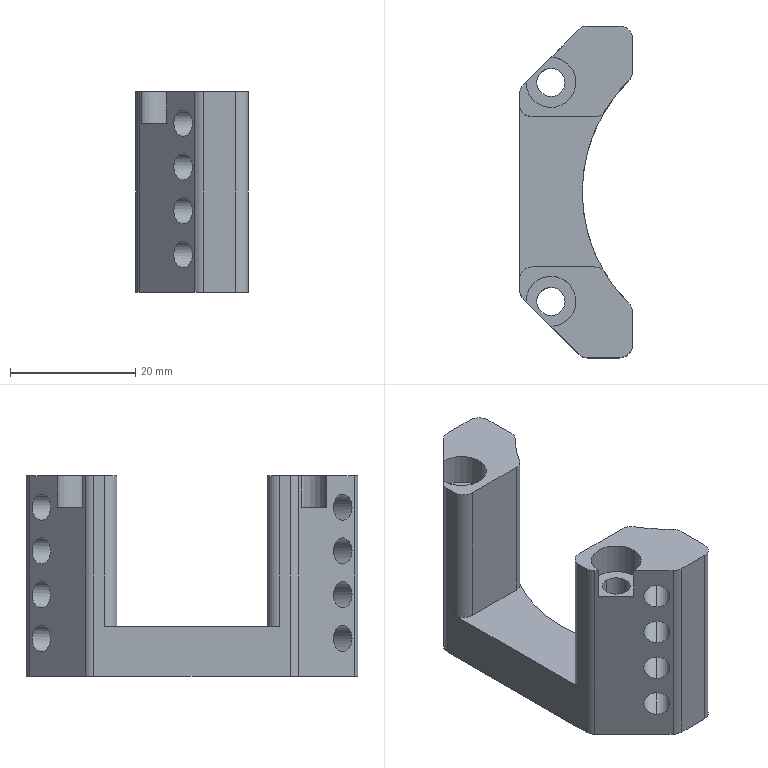NC program | Mastercam | posted with a generic post
Lines 42 to 1196 of 15624:
N430 T11 M6
N440 G0 G90 G17 G54 X-30.233 Y-26.319 A0. S7000 M3
N450 G43 H11 Z50. M8
N460 Z-22.696
N470 G1 Z-23.196 F600.
N480 X-30.432 Y-26.384 Z-23.233 F3000.
N490 X-30.636 Y-26.427 Z-23.27
N500 X-30.845 Y-26.449 Z-23.307
N510 X-31.054 Y-26.45 Z-23.344
N520 X-31.262 Y-26.428 Z-23.381
N530 X-31.467 Y-26.385 Z-23.418
N540 X-31.666 Y-26.32 Z-23.455
N550 X-31.857 Y-26.235 Z-23.491
N560 X-32.039 Y-26.131 Z-23.528
N570 X-32.208 Y-26.008 Z-23.565
N580 X-32.364 Y-25.868 Z-23.602
N590 X-32.504 Y-25.713 Z-23.639
N600 X-32.628 Y-25.543 Z-23.676
N610 X-32.732 Y-25.362 Z-23.713
N620 X-32.818 Y-25.171 Z-23.75
N630 X-34.177 Y-21.641
N640 X-34.77 Y-20.101 Z-23.859
N650 X-35.126 Y-19.176 Z-23.925
N660 X-35.216 Y-18.969 Z-23.94
N670 X-35.323 Y-18.77 Z-23.955
N680 X-35.446 Y-18.581 Z-23.97
N690 X-35.584 Y-18.403 Z-23.985
N700 X-35.737 Y-18.237 Z-24.
N710 X-36.107 Y-17.652
N720 X-36.389 Y-17.059
N730 X-36.616 Y-16.495
N740 X-36.796 Y-15.975
N750 X-36.934 Y-15.496
N760 X-37.037 Y-15.056
N770 X-37.114 Y-14.652
N780 X-37.171 Y-14.279
N790 X-37.247 Y-13.624
N800 X-37.292 Y-13.033
N810 X-37.319 Y-12.488
N820 X-37.336 Y-11.975
N830 X-37.345 Y-11.486
N840 X-37.35 Y-11.012
N850 X-37.352 Y-10.549
N860 Y-10.093
N870 X-37.351 Y-9.642
N880 X-37.349 Y-9.195
N890 X-37.347 Y-8.749
N900 X-37.345 Y-8.304
N910 X-37.342 Y-7.86
N920 X-37.34 Y-7.416
N930 X-37.337 Y-6.972
N940 X-37.334 Y-6.528
N950 X-37.332 Y-6.085
N960 X-37.329 Y-5.641
N970 X-37.326 Y-5.197
N980 X-37.323 Y-4.753
N990 X-37.32 Y-4.309
N1000 X-37.318 Y-3.866
N1010 X-37.315 Y-3.421
N1020 X-37.312 Y-2.977
N1030 X-37.309 Y-2.533
N1040 X-37.306 Y-2.089
N1050 X-37.304 Y-1.644
N1060 X-37.301 Y-1.2
N1070 X-37.298 Y-.756
N1080 X-37.295 Y-.311
N1090 X-37.292 Y.134
N1100 X-37.289 Y.578
N1110 X-37.287 Y1.023
N1120 X-37.284 Y1.468
N1130 X-37.281 Y1.913
N1140 X-37.278 Y2.358
N1150 X-37.275 Y2.803
N1160 X-37.272 Y3.248
N1170 X-37.27 Y3.694
N1180 X-37.267 Y4.139
N1190 X-37.264 Y4.584
N1200 X-37.261 Y5.03
N1210 X-37.258 Y5.475
N1220 X-37.256 Y5.921
N1230 X-37.253 Y6.366
N1240 X-37.25 Y6.812
N1250 X-37.247 Y7.258
N1260 X-37.244 Y7.703
N1270 X-37.241 Y8.149
N1280 X-37.239 Y8.595
N1290 X-37.236 Y9.041
N1300 X-37.233 Y9.487
N1310 X-37.23 Y9.933
N1320 X-37.227 Y10.379
N1330 X-37.224 Y10.825
N1340 X-37.222 Y11.271
N1350 X-37.219 Y11.717
N1360 X-37.216 Y12.167
N1370 X-37.18 Y12.772
N1380 X-37.078 Y13.384
N1390 X-36.911 Y13.987
N1400 X-36.685 Y14.57
N1410 X-36.405 Y15.123
N1420 X-36.08 Y15.639
N1430 X-35.72 Y16.113
N1440 X-35.333 Y16.544
N1450 X-34.928 Y16.93
N1460 X-34.512 Y17.273
N1470 X-34.092 Y17.576
N1480 X-33.672 Y17.84
N1490 X-33.256 Y18.071
N1500 X-32.848 Y18.271
N1510 X-32.449 Y18.444
N1520 X-32.061 Y18.593
N1530 X-31.685 Y18.722
N1540 X-31.319 Y18.833
N1550 X-30.966 Y18.929
N1560 X-30.304 Y19.08
N1570 X-29.676 Y19.196
N1580 X-29.078 Y19.284
N1590 X-28.507 Y19.351
N1600 X-27.958 Y19.402
N1610 X-27.428 Y19.441
N1620 X-26.913 Y19.471
N1630 X-26.411 Y19.494
N1640 X-25.92 Y19.511
N1650 X-25.437 Y19.524
N1660 X-24.961 Y19.534
N1670 X-24.491 Y19.54
N1680 X-24.025 Y19.545
N1690 X-23.563 Y19.548
N1700 X-23.105 Y19.55
N1710 X-22.648
N1720 X-22.194
N1730 X-21.741 Y19.549
N1740 X-21.289 Y19.548
N1750 X-20.838 Y19.546
N1760 X-20.388 Y19.544
N1770 X-19.938 Y19.542
N1780 X-19.489 Y19.539
N1790 X-19.04 Y19.537
N1800 X-18.591 Y19.534
N1810 X-18.142 Y19.532
N1820 X-17.693 Y19.529
N1830 X-17.245 Y19.526
N1840 X-16.796 Y19.523
N1850 X-16.347 Y19.521
N1860 X-15.899 Y19.518
N1870 X-15.45 Y19.515
N1880 X-15.002 Y19.512
N1890 X-14.553 Y19.509
N1900 X-14.104 Y19.506
N1910 X-13.656 Y19.504
N1920 X-13.207 Y19.501
N1930 X-12.759 Y19.498
N1940 X-12.31 Y19.495
N1950 X-11.861 Y19.492
N1960 X-11.413 Y19.489
N1970 X-10.964 Y19.487
N1980 X-10.515 Y19.484
N1990 X-10.066 Y19.481
N2000 X-9.618 Y19.478
N2010 X-9.169 Y19.475
N2020 X-8.72 Y19.472
N2030 X-8.271 Y19.47
N2040 X-7.822 Y19.467
N2050 X-7.373 Y19.464
N2060 X-6.925 Y19.461
N2070 X-6.476 Y19.458
N2080 X-6.027 Y19.455
N2090 X-5.578 Y19.452
N2100 X-5.129 Y19.45
N2110 X-4.68 Y19.447
N2120 X-4.231 Y19.444
N2130 X-3.782 Y19.441
N2140 X-3.333 Y19.438
N2150 X-2.884 Y19.435
N2160 X-2.435 Y19.433
N2170 X-1.986 Y19.43
N2180 X-1.537 Y19.427
N2190 X-1.088 Y19.424
N2200 X-.638 Y19.421
N2210 X-.189 Y19.418
N2220 X.26 Y19.415
N2230 X.709 Y19.413
N2240 X1.158 Y19.41
N2250 X1.608 Y19.407
N2260 X2.057 Y19.404
N2270 X2.506 Y19.401
N2280 X2.955 Y19.398
N2290 X3.405 Y19.395
N2300 X3.854 Y19.393
N2310 X4.303 Y19.39
N2320 X4.752 Y19.387
N2330 X5.202 Y19.384
N2340 X5.651 Y19.381
N2350 X6.101 Y19.378
N2360 X6.55 Y19.376
N2370 X6.999 Y19.373
N2380 X7.449 Y19.37
N2390 X7.898 Y19.367
N2400 X8.348 Y19.364
N2410 X8.797 Y19.361
N2420 X9.247 Y19.358
N2430 X9.696 Y19.356
N2440 X10.146 Y19.353
N2450 X10.595 Y19.35
N2460 X11.045 Y19.347
N2470 X11.494 Y19.344
N2480 X11.944 Y19.341
N2490 X12.393 Y19.338
N2500 X12.843 Y19.336
N2510 X13.293 Y19.333
N2520 X13.742 Y19.33
N2530 X14.192 Y19.327
N2540 X14.641 Y19.324
N2550 X15.091 Y19.321
N2560 X15.541 Y19.319
N2570 X15.991 Y19.316
N2580 X16.442 Y19.313
N2590 X16.894 Y19.311
N2600 X17.346 Y19.31
N2610 X17.798 Y19.308
N2620 X18.251 Y19.307
N2630 X18.705 Y19.306
N2640 X19.158 Y19.305
N2650 X19.612 Y19.304
N2660 X20.066
N2670 X20.52 Y19.303
N2680 X20.974
N2690 X21.429 Y19.302
N2700 X21.883
N2710 X22.338
N2720 X22.793 Y19.301
N2730 X23.248
N2740 X23.702
N2750 X24.157
N2760 X24.612
N2770 X25.067
N2780 X25.522
N2790 X25.977 Y19.3
N2800 X26.432
N2810 X26.887
N2820 X27.342
N2830 X27.797
N2840 X28.252
N2850 X28.733
N2860 X29.143 Y19.281
N2870 X29.564 Y19.229
N2880 X29.99 Y19.144
N2890 X30.418 Y19.026
N2900 X30.843 Y18.875
N2910 X31.26 Y18.692
N2920 X31.665 Y18.48
N2930 X32.055 Y18.242
N2940 X32.428 Y17.98
N2950 X32.782 Y17.698
N2960 X33.115 Y17.399
N2970 X33.427 Y17.086
N2980 X33.717 Y16.761
N2990 X33.986 Y16.429
N3000 X34.235 Y16.09
N3010 X34.463 Y15.748
N3020 X34.672 Y15.404
N3030 X34.863 Y15.06
N3040 X35.038 Y14.717
N3050 X35.196 Y14.376
N3060 X35.341 Y14.038
N3070 X35.472 Y13.703
N3080 X35.696 Y13.059
N3090 X35.881 Y12.431
N3100 X36.034 Y11.82
N3110 X36.161 Y11.226
N3120 X36.265 Y10.649
N3130 X36.352 Y10.086
N3140 X36.424 Y9.537
N3150 X36.484 Y9.001
N3160 X36.534 Y8.476
N3170 X36.576 Y7.96
N3180 X36.611 Y7.452
N3190 X36.641 Y6.953
N3200 X36.665 Y6.459
N3210 X36.686 Y5.971
N3220 X36.704 Y5.488
N3230 X36.718 Y5.009
N3240 X36.731 Y4.533
N3250 X36.741 Y4.06
N3260 X36.75 Y3.59
N3270 X36.758 Y3.122
N3280 X36.764 Y2.656
N3290 X36.77 Y2.192
N3300 X36.774 Y1.729
N3310 X36.778 Y1.267
N3320 X36.781 Y.806
N3330 X36.784 Y.346
N3340 X36.787 Y-.113
N3350 X36.789 Y-.572
N3360 X36.79 Y-1.03
N3370 X36.792 Y-1.487
N3380 X36.793 Y-1.945
N3390 X36.794 Y-2.402
N3400 X36.795 Y-2.858
N3410 X36.796 Y-3.315
N3420 Y-3.771
N3430 X36.797 Y-4.227
N3440 Y-4.683
N3450 X36.798 Y-5.139
N3460 Y-5.595
N3470 Y-6.05
N3480 X36.799 Y-6.506
N3490 Y-6.961
N3500 Y-7.417
N3510 Y-7.872
N3520 Y-8.328
N3530 Y-8.783
N3540 Y-9.238
N3550 X36.8 Y-9.694
N3560 Y-10.149
N3570 Y-10.604
N3580 Y-11.059
N3590 X36.796 Y-11.378
N3600 X36.766 Y-11.792
N3610 X36.702 Y-12.216
N3620 X36.605 Y-12.643
N3630 X36.475 Y-13.07
N3640 X36.312 Y-13.493
N3650 X36.119 Y-13.906
N3660 X35.898 Y-14.306
N3670 X35.651 Y-14.69
N3680 X35.381 Y-15.057
N3690 X35.093 Y-15.403
N3700 X34.788 Y-15.729
N3710 X34.471 Y-16.033
N3720 X34.143 Y-16.316
N3730 X33.808 Y-16.577
N3740 X33.468 Y-16.818
N3750 X33.125 Y-17.04
N3760 X32.781 Y-17.242
N3770 X32.437 Y-17.427
N3780 X32.094 Y-17.596
N3790 X31.754 Y-17.75
N3800 X31.418 Y-17.889
N3810 X31.085 Y-18.016
N3820 X30.443 Y-18.232
N3830 X29.818 Y-18.411
N3840 X29.211 Y-18.559
N3850 X28.62 Y-18.681
N3860 X28.045 Y-18.782
N3870 X27.485 Y-18.866
N3880 X26.938 Y-18.936
N3890 X26.404 Y-18.994
N3900 X25.881 Y-19.043
N3910 X25.366 Y-19.083
N3920 X24.86 Y-19.117
N3930 X24.362 Y-19.145
N3940 X23.869 Y-19.169
N3950 X23.382 Y-19.189
N3960 X22.9 Y-19.206
N3970 X22.421 Y-19.221
N3980 X21.946 Y-19.233
N3990 X21.474 Y-19.243
N4000 X21.004 Y-19.252
N4010 X20.537 Y-19.259
N4020 X20.071 Y-19.265
N4030 X19.607 Y-19.27
N4040 X19.144 Y-19.275
N4050 X18.683 Y-19.279
N4060 X18.222 Y-19.282
N4070 X17.762 Y-19.285
N4080 X17.303 Y-19.287
N4090 X16.845 Y-19.289
N4100 X16.386 Y-19.291
N4110 X15.929 Y-19.292
N4120 X15.472 Y-19.293
N4130 X15.015 Y-19.294
N4140 X14.558 Y-19.295
N4150 X14.102 Y-19.296
N4160 X13.645
N4170 X13.189 Y-19.297
N4180 X12.733
N4190 X12.278 Y-19.298
N4200 X11.822
N4210 X11.366
N4220 X10.911 Y-19.299
N4230 X10.455
N4240 X10.
N4250 X9.544
N4260 X9.089
N4270 X8.634
N4280 X8.178
N4290 X7.723 Y-19.3
N4300 X7.268
N4310 X6.812
N4320 X6.357
N4330 X5.902
N4340 X5.447
N4350 X4.992
N4360 X4.536
N4370 X4.081
N4380 X3.626
N4390 X3.171
N4400 X2.716
N4410 X2.261
N4420 X1.805
N4430 X1.35
N4440 X.895
N4450 X.44
N4460 X-.015
N4470 X-.47
N4480 X-.926
N4490 X-1.381
N4500 X-1.836
N4510 X-2.291
N4520 X-2.746
N4530 X-3.201
N4540 X-3.656
N4550 X-4.112
N4560 X-4.567
N4570 X-5.022
N4580 X-5.477
N4590 X-5.932
N4600 X-6.387
N4610 X-6.843
N4620 X-7.298
N4630 X-7.753
N4640 X-8.208
N4650 X-8.663
N4660 X-9.118
N4670 X-9.573
N4680 X-10.029
N4690 X-10.484
N4700 X-10.939
N4710 X-11.394
N4720 X-11.849
N4730 X-12.304
N4740 X-12.759
N4750 X-13.215
N4760 X-13.67
N4770 X-14.125
N4780 X-14.58
N4790 X-15.035
N4800 X-15.49
N4810 X-15.945
N4820 X-16.401
N4830 X-16.856
N4840 X-17.311
N4850 X-17.766
N4860 X-18.221
N4870 X-18.676
N4880 X-19.131
N4890 X-19.587
N4900 X-20.042
N4910 X-20.497
N4920 X-20.952
N4930 X-21.407
N4940 X-21.862
N4950 X-22.317
N4960 X-22.773
N4970 X-23.228
N4980 X-23.683
N4990 X-24.138
N5000 X-24.593
N5010 X-25.048
N5020 X-25.503
N5030 X-25.959
N5040 X-26.414
N5050 X-26.869
N5060 X-27.324
N5070 X-27.779
N5080 X-28.234
N5090 X-28.607 Y-19.293
N5100 X-29.05 Y-19.255
N5110 X-29.492 Y-19.184
N5120 X-29.931 Y-19.081
N5130 X-30.365 Y-18.947
N5140 X-30.791 Y-18.782
N5150 X-31.205 Y-18.588
N5160 X-31.606 Y-18.367
N5170 X-31.99 Y-18.123
N5180 X-32.357 Y-17.856
N5190 X-32.704 Y-17.571
N5200 X-33.031 Y-17.269
N5210 X-33.337 Y-16.955
N5220 X-33.622 Y-16.629
N5230 X-33.886 Y-16.297
N5240 X-34.13 Y-15.958
N5250 X-34.354 Y-15.616
N5260 X-34.56 Y-15.272
N5270 X-34.748 Y-14.927
N5280 X-34.92 Y-14.584
N5290 X-35.076 Y-14.243
N5300 X-35.218 Y-13.904
N5310 X-35.347 Y-13.57
N5320 X-35.567 Y-12.925
N5330 X-35.749 Y-12.296
N5340 X-35.898 Y-11.684
N5350 X-36.021 Y-11.089
N5360 X-36.123 Y-10.511
N5370 X-36.207 Y-9.947
N5380 X-36.275 Y-9.398
N5390 X-36.332 Y-8.861
N5400 X-36.379 Y-8.335
N5410 X-36.418 Y-7.819
N5420 X-36.45 Y-7.311
N5430 X-36.476 Y-6.811
N5440 X-36.498 Y-6.317
N5450 X-36.516 Y-5.829
N5460 X-36.53 Y-5.345
N5470 X-36.542 Y-4.866
N5480 X-36.551 Y-4.39
N5490 X-36.559 Y-3.917
N5500 X-36.565 Y-3.447
N5510 X-36.57 Y-2.979
N5520 X-36.573 Y-2.513
N5530 X-36.576 Y-2.049
N5540 X-36.577 Y-1.586
N5550 X-36.578 Y-1.124
N5560 X-36.579 Y-.663
N5570 X-36.578 Y-.203
N5580 Y.256
N5590 X-36.577 Y.715
N5600 X-36.576 Y1.173
N5610 X-36.574 Y1.631
N5620 X-36.573 Y2.088
N5630 X-36.571 Y2.545
N5640 X-36.569 Y3.002
N5650 X-36.567 Y3.458
N5660 X-36.565 Y3.915
N5670 X-36.562 Y4.371
N5680 X-36.56 Y4.827
N5690 X-36.557 Y5.283
N5700 X-36.555 Y5.738
N5710 X-36.552 Y6.194
N5720 X-36.55 Y6.649
N5730 X-36.547 Y7.105
N5740 X-36.544 Y7.56
N5750 X-36.541 Y8.016
N5760 X-36.539 Y8.471
N5770 X-36.536 Y8.927
N5780 X-36.532 Y9.431
N5790 X-36.516 Y9.842
N5800 X-36.479 Y10.275
N5810 X-36.418 Y10.714
N5820 X-36.331 Y11.152
N5830 X-36.219 Y11.587
N5840 X-36.082 Y12.014
N5850 X-35.92 Y12.433
N5860 X-35.736 Y12.84
N5870 X-35.529 Y13.235
N5880 X-35.302 Y13.617
N5890 X-35.057 Y13.98
N5900 X-34.795 Y14.33
N5910 X-34.519 Y14.66
N5920 X-34.229 Y14.975
N5930 X-33.929 Y15.27
N5940 X-33.62 Y15.549
N5950 X-33.303 Y15.81
N5960 X-32.981 Y16.054
N5970 X-32.655 Y16.28
N5980 X-32.325 Y16.491
N5990 X-31.995 Y16.686
N6000 X-31.663 Y16.866
N6010 X-31.332 Y17.033
N6020 X-31.003 Y17.186
N6030 X-30.675 Y17.327
N6040 X-30.038 Y17.572
N6050 X-29.413 Y17.778
N6060 X-28.799 Y17.952
N6070 X-28.2 Y18.098
N6080 X-27.614 Y18.22
N6090 X-27.042 Y18.322
N6100 X-26.482 Y18.407
N6110 X-25.935 Y18.479
N6120 X-25.398 Y18.538
N6130 X-24.872 Y18.587
N6140 X-24.355 Y18.629
N6150 X-23.846 Y18.663
N6160 X-23.344 Y18.691
N6170 X-22.848 Y18.715
N6180 X-22.358 Y18.734
N6190 X-21.873 Y18.75
N6200 X-21.392 Y18.763
N6210 X-20.915 Y18.774
N6220 X-20.441 Y18.782
N6230 X-19.97 Y18.789
N6240 X-19.501 Y18.794
N6250 X-19.034 Y18.798
N6260 X-18.569 Y18.801
N6270 X-18.105 Y18.803
N6280 X-17.643 Y18.805
N6290 X-17.181
N6300 X-16.721 Y18.806
N6310 X-16.261 Y18.805
N6320 X-15.802
N6330 X-15.344 Y18.804
N6340 X-14.886 Y18.802
N6350 X-14.428 Y18.801
N6360 X-13.971 Y18.799
N6370 X-13.514 Y18.797
N6380 X-13.057 Y18.795
N6390 X-12.601 Y18.793
N6400 X-12.145 Y18.791
N6410 X-11.689 Y18.788
N6420 X-11.233 Y18.786
N6430 X-10.777 Y18.783
N6440 X-10.321 Y18.781
N6450 X-9.866 Y18.778
N6460 X-9.41 Y18.775
N6470 X-8.955 Y18.773
N6480 X-8.499 Y18.77
N6490 X-8.044 Y18.767
N6500 X-7.589 Y18.765
N6510 X-7.133 Y18.762
N6520 X-6.678 Y18.759
N6530 X-6.223 Y18.756
N6540 X-5.767 Y18.753
N6550 X-5.312 Y18.75
N6560 X-4.857 Y18.748
N6570 X-4.402 Y18.745
N6580 X-3.947 Y18.742
N6590 X-3.491 Y18.739
N6600 X-3.036 Y18.736
N6610 X-2.581 Y18.733
N6620 X-2.126 Y18.73
N6630 X-1.671 Y18.728
N6640 X-1.216 Y18.725
N6650 X-.76 Y18.722
N6660 X-.305 Y18.719
N6670 X.15 Y18.716
N6680 X.605 Y18.713
N6690 X1.06 Y18.71
N6700 X1.515 Y18.707
N6710 X1.97 Y18.705
N6720 X2.426 Y18.702
N6730 X2.881 Y18.699
N6740 X3.336 Y18.696
N6750 X3.791 Y18.693
N6760 X4.246 Y18.69
N6770 X4.701 Y18.687
N6780 X5.156 Y18.684
N6790 X5.612 Y18.681
N6800 X6.067 Y18.679
N6810 X6.522 Y18.676
N6820 X6.977 Y18.673
N6830 X7.432 Y18.67
N6840 X7.887 Y18.667
N6850 X8.342 Y18.664
N6860 X8.798 Y18.661
N6870 X9.253 Y18.658
N6880 X9.708 Y18.655
N6890 X10.163 Y18.653
N6900 X10.618 Y18.65
N6910 X11.073 Y18.647
N6920 X11.528 Y18.644
N6930 X11.984 Y18.641
N6940 X12.439 Y18.638
N6950 X12.894 Y18.635
N6960 X13.348 Y18.632
N6970 X13.803 Y18.63
N6980 X14.256 Y18.627
N6990 X14.71 Y18.624
N7000 X15.163 Y18.622
N7010 X15.617 Y18.62
N7020 X16.07 Y18.618
N7030 X16.523 Y18.616
N7040 X16.977 Y18.614
N7050 X17.43 Y18.613
N7060 X17.884 Y18.611
N7070 X18.337 Y18.61
N7080 X18.791 Y18.609
N7090 X19.245 Y18.608
N7100 X19.699 Y18.607
N7110 X20.153 Y18.606
N7120 X20.607 Y18.605
N7130 X21.062
N7140 X21.516 Y18.604
N7150 X21.971
N7160 X22.425 Y18.603
N7170 X22.88
N7180 X23.334 Y18.602
N7190 X23.789
N7200 X24.244
N7210 X24.699
N7220 X25.154 Y18.601
N7230 X25.609
N7240 X26.238 Y18.593
N7250 X26.659 Y18.565
N7260 X27.087 Y18.517
N7270 X27.518 Y18.445
N7280 X27.946 Y18.351
N7290 X28.369 Y18.234
N7300 X28.786 Y18.094
N7310 X29.193 Y17.934
N7320 X29.59 Y17.753
N7330 X29.976 Y17.552
N7340 X30.348 Y17.333
N7350 X30.706 Y17.099
N7360 X31.048 Y16.85
N7370 X31.377 Y16.587
N7380 X31.688 Y16.314
N7390 X31.985 Y16.029
N7400 X32.265 Y15.737
N7410 X32.531 Y15.436
N7420 X32.781 Y15.131
N7430 X33.016 Y14.82
N7440 X33.236 Y14.506
N7450 X33.442 Y14.189
N7460 X33.634 Y13.871
N7470 X33.814 Y13.551
N7480 X33.981 Y13.233
N7490 X34.137 Y12.914
N7500 X34.412 Y12.292
N7510 X34.649 Y11.677
N7520 X34.853 Y11.071
N7530 X35.029 Y10.474
N7540 X35.18 Y9.888
N7550 X35.309 Y9.313
N7560 X35.42 Y8.749
N7570 X35.516 Y8.196
N7580 X35.597 Y7.652
N7590 X35.667 Y7.118
N7600 X35.727 Y6.593
N7610 X35.779 Y6.075
N7620 X35.823 Y5.564
N7630 X35.862 Y5.06
N7640 X35.894 Y4.562
N7650 X35.923 Y4.069
N7660 X35.947 Y3.581
N7670 X35.968 Y3.097
N7680 X35.986 Y2.616
N7690 X36.002 Y2.138
N7700 X36.015 Y1.664
N7710 X36.027 Y1.192
N7720 X36.037 Y.722
N7730 X36.045 Y.254
N7740 X36.053 Y-.213
N7750 X36.059 Y-.677
N7760 X36.065 Y-1.141
N7770 X36.07 Y-1.604
N7780 X36.074 Y-2.065
N7790 X36.078 Y-2.526
N7800 X36.081 Y-2.986
N7810 X36.083 Y-3.445
N7820 X36.086 Y-3.904
N7830 X36.088 Y-4.362
N7840 X36.089 Y-4.82
N7850 X36.091 Y-5.277
N7860 X36.092 Y-5.735
N7870 X36.093 Y-6.191
N7880 X36.094 Y-6.648
N7890 X36.095 Y-7.105
N7900 X36.096 Y-7.561
N7910 Y-8.017
N7920 X36.093 Y-8.586
N7930 X36.074 Y-9.001
N7940 X36.033 Y-9.428
N7950 X35.97 Y-9.859
N7960 X35.885 Y-10.288
N7970 X35.776 Y-10.714
N7980 X35.645 Y-11.133
N7990 X35.492 Y-11.544
N8000 X35.318 Y-11.945
N8010 X35.125 Y-12.335
N8020 X34.912 Y-12.713
N8030 X34.684 Y-13.076
N8040 X34.44 Y-13.425
N8050 X34.183 Y-13.757
N8060 X33.912 Y-14.076
N8070 X33.632 Y-14.378
N8080 X33.342 Y-14.665
N8090 X33.045 Y-14.936
N8100 X32.74 Y-15.192
N8110 X32.432 Y-15.432
N8120 X32.118 Y-15.658
N8130 X31.802 Y-15.869
N8140 X31.484 Y-16.066
N8150 X31.166 Y-16.25
N8160 X30.846 Y-16.422
N8170 X30.528 Y-16.582
N8180 X30.21 Y-16.73
N8190 X29.59 Y-16.992
N8200 X28.977 Y-17.218
N8210 X28.374 Y-17.413
N8220 X27.781 Y-17.58
N8230 X27.198 Y-17.724
N8240 X26.627 Y-17.847
N8250 X26.066 Y-17.953
N8260 X25.516 Y-18.043
N8270 X24.976 Y-18.121
N8280 X24.444 Y-18.188
N8290 X23.921 Y-18.245
N8300 X23.406 Y-18.294
N8310 X22.898 Y-18.336
N8320 X22.396 Y-18.373
N8330 X21.899 Y-18.404
N8340 X21.408 Y-18.431
N8350 X20.921 Y-18.454
N8360 X20.438 Y-18.474
N8370 X19.958 Y-18.491
N8380 X19.482 Y-18.506
N8390 X19.008 Y-18.519
N8400 X18.537 Y-18.53
N8410 X18.067 Y-18.54
N8420 X17.6 Y-18.548
N8430 X17.134 Y-18.555
N8440 X16.67 Y-18.561
N8450 X16.206 Y-18.567
N8460 X15.744 Y-18.571
N8470 X15.283 Y-18.575
N8480 X14.823 Y-18.579
N8490 X14.363 Y-18.582
N8500 X13.904 Y-18.584
N8510 X13.445 Y-18.586
N8520 X12.987 Y-18.588
N8530 X12.529 Y-18.59
N8540 X12.072 Y-18.591
N8550 X11.615 Y-18.592
N8560 X11.158 Y-18.593
N8570 X10.701 Y-18.594
N8580 X10.245 Y-18.595
N8590 X9.789 Y-18.596
N8600 X9.333
N8610 X8.877 Y-18.597
N8620 X8.421
N8630 X7.965 Y-18.598
N8640 X7.51
N8650 X7.054
N8660 X6.598 Y-18.599
N8670 X6.143
N8680 X5.688
N8690 X5.232
N8700 X4.777
N8710 X4.321
N8720 X3.866
N8730 X3.411
N8740 X2.956 Y-18.6
N8750 X2.5
N8760 X2.045
N8770 X1.59
N8780 X1.135
N8790 X.679
N8800 X.224
N8810 X-.231
N8820 X-.686
N8830 X-1.141
N8840 X-1.596
N8850 X-2.052
N8860 X-2.507
N8870 X-2.962
N8880 X-3.417
N8890 X-3.872
N8900 X-4.327
N8910 X-4.783
N8920 X-5.238
N8930 X-5.693
N8940 X-6.148
N8950 X-6.603
N8960 X-7.058
N8970 X-7.514
N8980 X-7.969
N8990 X-8.424
N9000 X-8.879
N9010 X-9.334
N9020 X-9.789
N9030 X-10.244
N9040 X-10.7
N9050 X-11.155
N9060 X-11.61
N9070 X-12.065
N9080 X-12.52
N9090 X-12.975
N9100 X-13.43
N9110 X-13.886
N9120 X-14.341
N9130 X-14.796
N9140 X-15.251
N9150 X-15.706
N9160 X-16.161
N9170 X-16.616
N9180 X-17.072
N9190 X-17.527
N9200 X-17.982
N9210 X-18.437
N9220 X-18.892
N9230 X-19.347
N9240 X-19.802
N9250 X-20.258
N9260 X-20.713
N9270 X-21.168
N9280 X-21.623
N9290 X-22.078
N9300 X-22.533
N9310 X-22.988
N9320 X-23.444
N9330 X-23.899
N9340 X-24.354
N9350 X-24.809
N9360 X-25.264
N9370 X-25.834 Y-18.596
N9380 X-26.235 Y-18.578
N9390 X-26.654 Y-18.54
N9400 X-27.079 Y-18.482
N9410 X-27.505 Y-18.401
N9420 X-27.929 Y-18.298
N9430 X-28.348 Y-18.173
N9440 X-28.759 Y-18.026
N9450 X-29.162 Y-17.859
N9460 X-29.553 Y-17.671
N9470 X-29.934 Y-17.465
N9480 X-30.301 Y-17.241
N9490 X-30.653 Y-17.002
N9500 X-30.99 Y-16.749
N9510 X-31.313 Y-16.483
N9520 X-31.62 Y-16.207
N9530 X-31.912 Y-15.92
N9540 X-32.187 Y-15.625
N9550 X-32.448 Y-15.323
N9560 X-32.692 Y-15.016
N9570 X-32.924 Y-14.703
N9580 X-33.139 Y-14.389
N9590 X-33.341 Y-14.07
N9600 X-33.53 Y-13.752
N9610 X-33.706 Y-13.431
N9620 X-33.869 Y-13.112
N9630 X-34.022 Y-12.793
N9640 X-34.29 Y-12.17
N9650 X-34.521 Y-11.555
N9660 X-34.72 Y-10.948
N9670 X-34.891 Y-10.351
N9680 X-35.038 Y-9.765
N9690 X-35.163 Y-9.19
N9700 X-35.27 Y-8.626
N9710 X-35.361 Y-8.072
N9720 X-35.439 Y-7.529
N9730 X-35.505 Y-6.995
N9740 X-35.562 Y-6.469
N9750 X-35.61 Y-5.951
N9760 X-35.651 Y-5.441
N9770 X-35.686 Y-4.937
N9780 X-35.716 Y-4.438
N9790 X-35.741 Y-3.945
N9800 X-35.762 Y-3.457
N9810 X-35.78 Y-2.973
N9820 X-35.795 Y-2.492
N9830 X-35.807 Y-2.014
N9840 X-35.818 Y-1.54
N9850 X-35.827 Y-1.068
N9860 X-35.834 Y-.598
N9870 X-35.839 Y-.13
N9880 X-35.844 Y.337
N9890 X-35.847 Y.802
N9900 X-35.85 Y1.265
N9910 X-35.852 Y1.728
N9920 X-35.853 Y2.189
N9930 X-35.854 Y2.65
N9940 Y3.11
N9950 Y3.569
N9960 X-35.853 Y4.028
N9970 X-35.852 Y4.486
N9980 X-35.851 Y4.944
N9990 X-35.85 Y5.402
N100 X-35.848 Y5.859
N110 X-35.846 Y6.316
N120 X-35.844 Y6.794
N130 X-35.831 Y7.381
N140 X-35.814 Y7.729
N150 X-35.784 Y8.101
N160 X-35.74 Y8.489
N170 X-35.678 Y8.887
N180 X-35.599 Y9.288
N190 X-35.501 Y9.692
N200 X-35.384 Y10.094
N210 X-35.248 Y10.491
N220 X-35.094 Y10.883
N230 X-34.922 Y11.266
N240 X-34.733 Y11.64
N250 X-34.528 Y12.004
N260 X-34.307 Y12.359
N270 X-34.072 Y12.7
N280 X-33.825 Y13.027
N290 X-33.567 Y13.34
N300 X-33.298 Y13.641
N310 X-33.021 Y13.927
N320 X-32.734 Y14.201
N330 X-32.442 Y14.458
N340 X-32.143 Y14.705
N350 X-31.84 Y14.935
N360 X-31.532 Y15.154
N370 X-31.223 Y15.359
N380 X-30.911 Y15.553
N390 X-30.598 Y15.733
N400 X-30.284 Y15.903
N410 X-29.97 Y16.061
N420 X-29.356 Y16.343
N430 X-28.745 Y16.589
N440 X-28.141 Y16.802
N450 X-27.545 Y16.987
N460 X-26.958 Y17.147
N470 X-26.381 Y17.285
N480 X-25.813 Y17.404
N490 X-25.256 Y17.506
N500 X-24.708 Y17.594
N510 X-24.169 Y17.669
N520 X-23.638 Y17.734
N530 X-23.116 Y17.789
N540 X-22.6 Y17.837
N550 X-22.092 Y17.877
N560 X-21.589 Y17.912
N570 X-21.092 Y17.941
N580 X-20.599 Y17.967
N590 X-20.111 Y17.988
N600 X-19.628 Y18.006
N610 X-19.147 Y18.021
N620 X-18.67 Y18.034
N630 X-18.195 Y18.045
N640 X-17.723 Y18.054
N650 X-17.253 Y18.061
N660 X-16.785 Y18.067
N670 X-16.318 Y18.071
N680 X-15.853 Y18.075
N690 X-15.389 Y18.078
N700 X-14.927 Y18.08
N710 X-14.465 Y18.081
N720 X-14.004 Y18.082
N730 X-13.544
N740 X-13.085
N750 X-12.626
N760 X-12.167 Y18.081
N770 X-11.709 Y18.08
N780 X-11.252 Y18.079
N790 X-10.795 Y18.077
N800 X-10.338 Y18.075
N810 X-9.881 Y18.073
N820 X-9.424 Y18.071
N830 X-8.968 Y18.069
N840 X-8.512 Y18.067
N850 X-8.056 Y18.065
N860 X-7.6 Y18.062
N870 X-7.144 Y18.06
N880 X-6.688 Y18.057
N890 X-6.233 Y18.055
N900 X-5.777 Y18.052
N910 X-5.322 Y18.049
N920 X-4.866 Y18.047
N930 X-4.411 Y18.044
N940 X-3.956 Y18.041
N950 X-3.5 Y18.038
N960 X-3.045 Y18.036
N970 X-2.59 Y18.033
N980 X-2.134 Y18.03
N990 X-1.679 Y18.027
N1000 X-1.224 Y18.024
N1010 X-.769 Y18.022
N1020 X-.313 Y18.019
N1030 X.142 Y18.016
N1040 X.597 Y18.013
N1050 X1.052 Y18.01
N1060 X1.507 Y18.007
N1070 X1.963 Y18.004
N1080 X2.418 Y18.002
N1090 X2.873 Y17.999
N1100 X3.328 Y17.996
N1110 X3.783 Y17.993
N1120 X4.238 Y17.99
N1130 X4.694 Y17.987
N1140 X5.149 Y17.984
N1150 X5.604 Y17.981
N1160 X6.059 Y17.979
N1170 X6.514 Y17.976
N1180 X6.969 Y17.973
N1190 X7.424 Y17.97
N1200 X7.88 Y17.967
N1210 X8.335 Y17.964
N1220 X8.79 Y17.961
N1230 X9.245 Y17.958
N1240 X9.7 Y17.956
N1250 X10.155 Y17.953
N1260 X10.61 Y17.95
N1270 X11.065 Y17.947
N1280 X11.52 Y17.944
N1290 X11.975 Y17.941
N1300 X12.429 Y17.938
N1310 X12.883 Y17.936
N1320 X13.338 Y17.933
N1330 X13.792 Y17.931
N1340 X14.246 Y17.928
N1350 X14.699 Y17.926
N1360 X15.153 Y17.924
N1370 X15.607 Y17.922
N1380 X16.061 Y17.92
N1390 X16.515 Y17.918
N1400 X16.968 Y17.917
N1410 X17.422 Y17.915
N1420 X17.876 Y17.914
N1430 X18.33 Y17.912
N1440 X18.784 Y17.911
N1450 X19.238 Y17.91
N1460 X19.692 Y17.909
N1470 X20.147 Y17.908
N1480 X20.601 Y17.907
N1490 X21.055
N1500 X21.51 Y17.906
N1510 X21.964 Y17.905
N1520 X22.419
N1530 X22.876 Y17.904
N1540 X23.351 Y17.903
N1550 X23.927 Y17.893
N1560 X24.598 Y17.857
N1570 X24.966 Y17.822
N1580 X25.346 Y17.772
N1590 X25.732 Y17.708
N1600 X26.123 Y17.627
N1610 X26.514 Y17.53
N1620 X26.905 Y17.415
N1630 X27.293 Y17.284
N1640 X27.674 Y17.136
N1650 X28.05 Y16.971
N1660 X28.418 Y16.791
N1670 X28.777 Y16.596
N1680 X29.125 Y16.387
N1690 X29.466 Y16.163
N1700 X29.79 Y15.93
N1710 X30.107 Y15.683
N1720 X30.408 Y15.428
N1730 X30.699 Y15.163
N1740 X30.976 Y14.89
N1750 X31.24 Y14.611
N1760 X31.493 Y14.324
N1770 X31.732 Y14.034
N1780 X31.959 Y13.737
N1790 X32.174 Y13.439
N1800 X32.378 Y13.137
N1810 X32.569 Y12.834
N1820 X32.751 Y12.527
N1830 X32.921 Y12.222
N1840 X33.228 Y11.62
N1850 X33.498 Y11.019
N1860 X33.737 Y10.422
N1870 X33.947 Y9.83
N1880 X34.131 Y9.245
N1890 X34.292 Y8.668
N1900 X34.433 Y8.1
N1910 X34.556 Y7.539
N1920 X34.663 Y6.988
N1930 X34.757 Y6.444
N1940 X34.838 Y5.909
N1950 X34.91 Y5.381
N1960 X34.972 Y4.859
N1970 X35.026 Y4.345
N1980 X35.074 Y3.836
N1990 X35.115 Y3.334
N2000 X35.151 Y2.836
N2010 X35.183 Y2.342
N2020 X35.21 Y1.853
N2030 X35.234 Y1.368
N2040 X35.255 Y.886
N2050 X35.274 Y.407
N2060 X35.29 Y-.069
N2070 X35.304 Y-.543